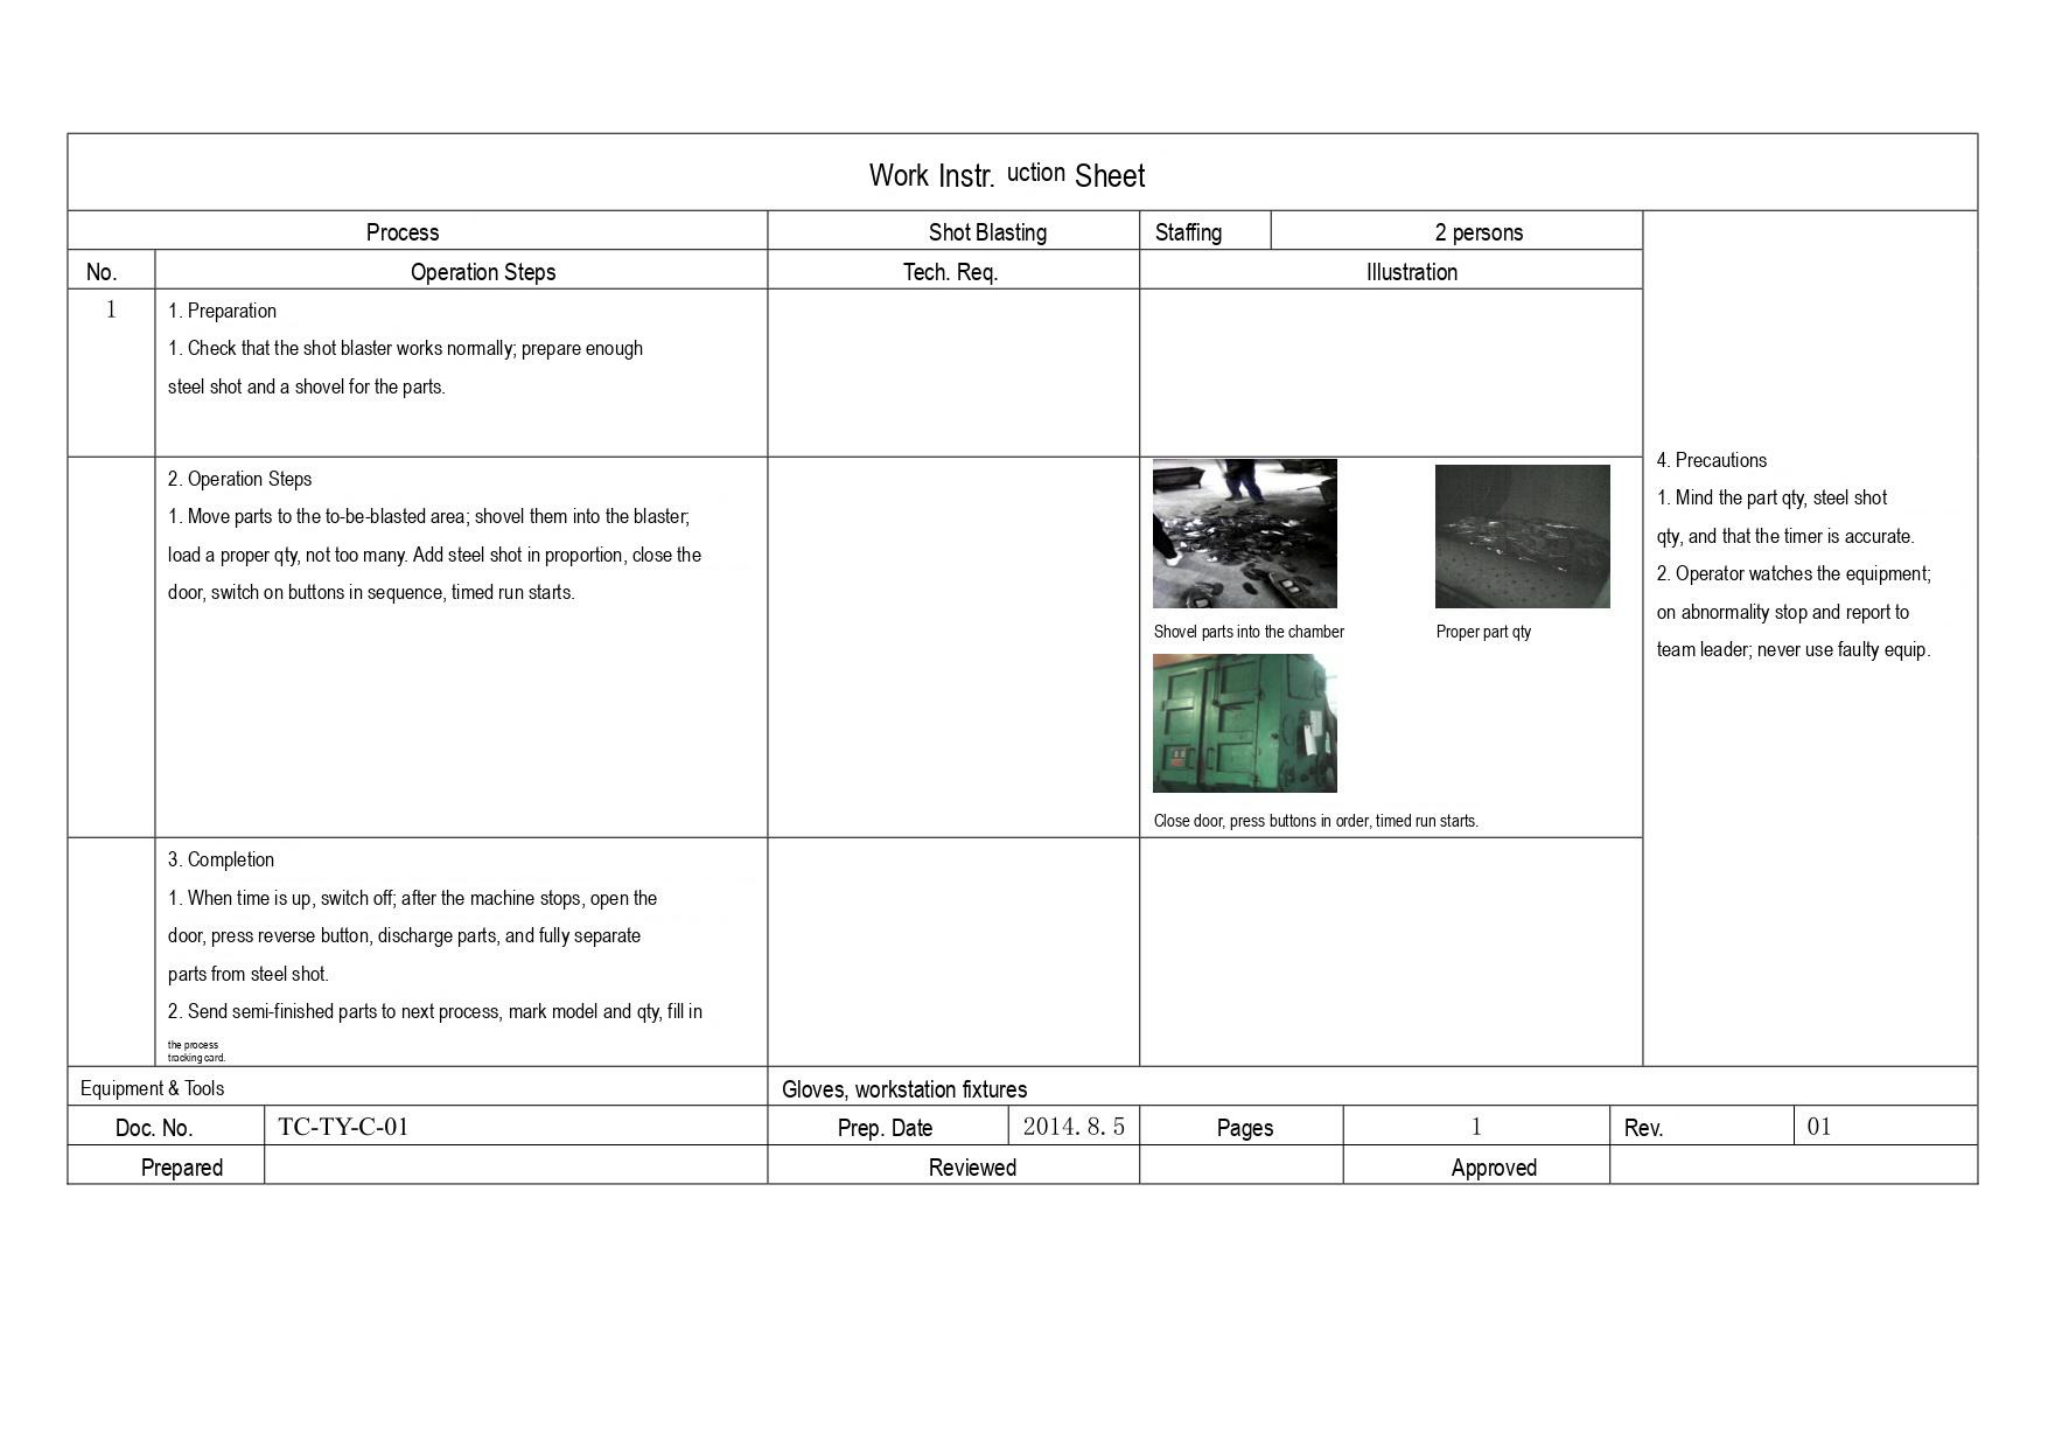Work Instr. uction Sheet

| Process | | Shot Blasting | Staffing | 2 persons | |
|---|---|---|---|---|---|
| **No.** | **Operation Steps** | **Tech. Req.** | **Illustration** | | 4. Precautions<br>1. Mind the part qty, steel shot qty, and that the timer is accurate.<br>2. Operator watches the equipment; on abnormality stop and report to team leader; never use faulty equip. |
| 1 | 1. Preparation<br>1. Check that the shot blaster works normally; prepare enough steel shot and a shovel for the parts. | | | | |
| | 2. Operation Steps<br>1. Move parts to the to-be-blasted area; shovel them into the blaster; load a proper qty, not too many. Add steel shot in proportion, close the door, switch on buttons in sequence, timed run starts. | | Shovel parts into the chamber<br>Proper part qty<br>Close door, press buttons in order, timed run starts. | | |
| | 3. Completion<br>1. When time is up, switch off; after the machine stops, open the door, press reverse button, discharge parts, and fully separate parts from steel shot.<br>2. Send semi-finished parts to next process, mark model and qty, fill in the process tracking card. | | | | |

| Equipment & Tools | | Gloves, workstation fixtures | | | | | |
|---|---|---|---|---|---|---|---|
| Doc. No. | TC-TY-C-01 | Prep. Date | 2014. 8. 5 | Pages | 1 | Rev. | 01 |
| Prepared | | Reviewed | | Approved | | | |